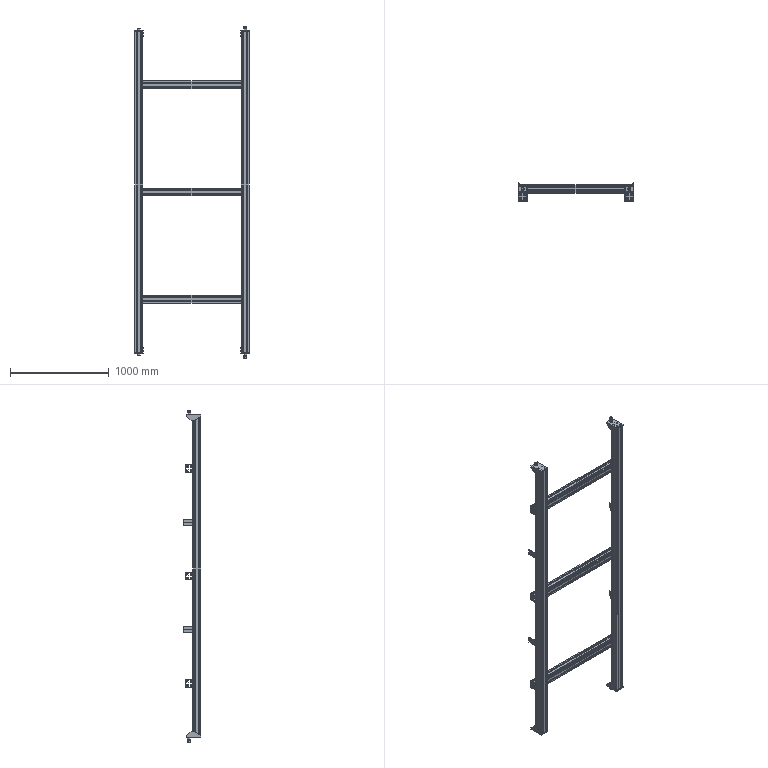Part | NX | features BREP 5 | 21 solids | 1006 faces | box 1173 x 180 x 3362 mm | volume 25641437 mm3 | plane 758 | cylinder 136 | cone 112 | commonest cylinder face diameters 6.8 x80 8.5 x32 20 x16 21 x8